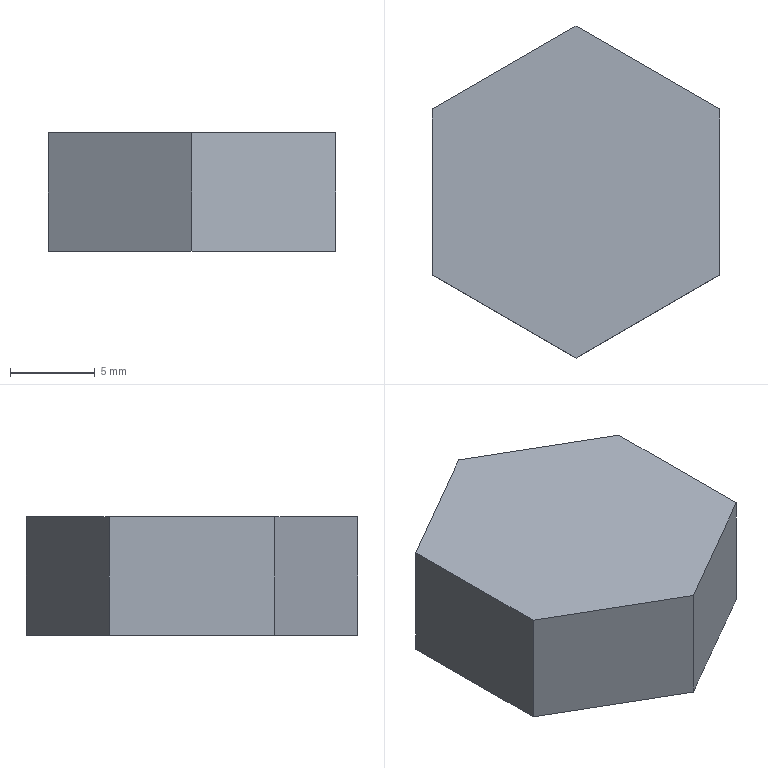Part | SolidWorks | features BaseBody 1 | 1 solid | 15 faces | box 17 x 19.63 x 7 mm | volume 818.394 mm3 | plane 15
STEP:
#1=CARTESIAN_POINT('',(-7.,-4.041,5.5));
#2=VERTEX_POINT('',#1);
#3=CARTESIAN_POINT('',(0.,-8.083,5.5));
#4=VERTEX_POINT('',#3);
#5=CARTESIAN_POINT('',(-7.75,-3.608,5.5));
#6=DIRECTION('',(0.866,-0.5,0.));
#7=VECTOR('',#6,1000.);
#8=LINE('',#5,#7);
#9=EDGE_CURVE('',#2,#4,#8,.T.);
#10=ORIENTED_EDGE('',*,*,#9,.F.);
#11=CARTESIAN_POINT('',(-7.,4.041,5.5));
#12=VERTEX_POINT('',#11);
#13=CARTESIAN_POINT('',(-7.,4.907,5.5));
#14=DIRECTION('',(0.,-1.,0.));
#15=VECTOR('',#14,1000.);
#16=LINE('',#13,#15);
#17=EDGE_CURVE('',#12,#2,#16,.T.);
#18=ORIENTED_EDGE('',*,*,#17,.F.);
#19=CARTESIAN_POINT('',(0.,8.083,5.5));
#20=VERTEX_POINT('',#19);
#21=CARTESIAN_POINT('',(0.75,8.516,5.5));
#22=DIRECTION('',(-0.866,-0.5,0.));
#23=VECTOR('',#22,1000.);
#24=LINE('',#21,#23);
#25=EDGE_CURVE('',#20,#12,#24,.T.);
#26=ORIENTED_EDGE('',*,*,#25,.F.);
#27=CARTESIAN_POINT('',(7.,4.041,5.5));
#28=VERTEX_POINT('',#27);
#29=CARTESIAN_POINT('',(7.75,3.608,5.5));
#30=DIRECTION('',(-0.866,0.5,0.));
#31=VECTOR('',#30,1000.);
#32=LINE('',#29,#31);
#33=EDGE_CURVE('',#28,#20,#32,.T.);
#34=ORIENTED_EDGE('',*,*,#33,.F.);
#35=CARTESIAN_POINT('',(7.,-4.041,5.5));
#36=VERTEX_POINT('',#35);
#37=CARTESIAN_POINT('',(7.,-4.907,5.5));
#38=DIRECTION('',(0.,1.,0.));
#39=VECTOR('',#38,1000.);
#40=LINE('',#37,#39);
#41=EDGE_CURVE('',#36,#28,#40,.T.);
#42=ORIENTED_EDGE('',*,*,#41,.F.);
#43=CARTESIAN_POINT('',(-0.75,-8.516,5.5));
#44=DIRECTION('',(0.866,0.5,0.));
#45=VECTOR('',#44,1000.);
#46=LINE('',#43,#45);
#47=EDGE_CURVE('',#4,#36,#46,.T.);
#48=ORIENTED_EDGE('',*,*,#47,.F.);
#49=EDGE_LOOP('',(#10,#18,#26,#34,#42,#48));
#50=FACE_OUTER_BOUND('',#49,.T.);
#51=CARTESIAN_POINT('',(0.,0.,5.5));
#52=DIRECTION('',(0.,0.,1.));
#53=DIRECTION('',(1.,0.,0.));
#54=AXIS2_PLACEMENT_3D('',#51,#52,#53);
#55=PLANE('',#54);
#56=ADVANCED_FACE('',(#50),#55,.F.);
#57=CARTESIAN_POINT('',(-7.,4.041,0.));
#58=VERTEX_POINT('',#57);
#59=CARTESIAN_POINT('',(-7.,-4.041,0.));
#60=VERTEX_POINT('',#59);
#61=CARTESIAN_POINT('',(-7.,4.907,0.));
#62=DIRECTION('',(0.,-1.,0.));
#63=VECTOR('',#62,1000.);
#64=LINE('',#61,#63);
#65=EDGE_CURVE('',#58,#60,#64,.T.);
#66=ORIENTED_EDGE('',*,*,#65,.F.);
#67=CARTESIAN_POINT('',(-7.,4.041,7.));
#68=DIRECTION('',(0.,0.,-1.));
#69=VECTOR('',#68,1000.);
#70=LINE('',#67,#69);
#71=EDGE_CURVE('',#12,#58,#70,.T.);
#72=ORIENTED_EDGE('',*,*,#71,.F.);
#73=ORIENTED_EDGE('',*,*,#17,.T.);
#74=CARTESIAN_POINT('',(-7.,-4.041,7.));
#75=DIRECTION('',(0.,0.,-1.));
#76=VECTOR('',#75,1000.);
#77=LINE('',#74,#76);
#78=EDGE_CURVE('',#2,#60,#77,.T.);
#79=ORIENTED_EDGE('',*,*,#78,.T.);
#80=EDGE_LOOP('',(#66,#72,#73,#79));
#81=FACE_OUTER_BOUND('',#80,.T.);
#82=CARTESIAN_POINT('',(-7.,4.907,7.));
#83=DIRECTION('',(1.,0.,0.));
#84=DIRECTION('',(0.,1.,0.));
#85=AXIS2_PLACEMENT_3D('',#82,#83,#84);
#86=PLANE('',#85);
#87=ADVANCED_FACE('',(#81),#86,.T.);
#88=CARTESIAN_POINT('',(0.,8.083,0.));
#89=VERTEX_POINT('',#88);
#90=CARTESIAN_POINT('',(0.75,8.516,0.));
#91=DIRECTION('',(-0.866,-0.5,0.));
#92=VECTOR('',#91,1000.);
#93=LINE('',#90,#92);
#94=EDGE_CURVE('',#89,#58,#93,.T.);
#95=ORIENTED_EDGE('',*,*,#94,.F.);
#96=CARTESIAN_POINT('',(0.,8.083,7.));
#97=DIRECTION('',(0.,0.,-1.));
#98=VECTOR('',#97,1000.);
#99=LINE('',#96,#98);
#100=EDGE_CURVE('',#20,#89,#99,.T.);
#101=ORIENTED_EDGE('',*,*,#100,.F.);
#102=ORIENTED_EDGE('',*,*,#25,.T.);
#103=ORIENTED_EDGE('',*,*,#71,.T.);
#104=EDGE_LOOP('',(#95,#101,#102,#103));
#105=FACE_OUTER_BOUND('',#104,.T.);
#106=CARTESIAN_POINT('',(0.75,8.516,7.));
#107=DIRECTION('',(0.5,-0.866,0.));
#108=DIRECTION('',(0.,0.,-1.));
#109=AXIS2_PLACEMENT_3D('',#106,#107,#108);
#110=PLANE('',#109);
#111=ADVANCED_FACE('',(#105),#110,.T.);
#112=CARTESIAN_POINT('',(7.,4.041,0.));
#113=VERTEX_POINT('',#112);
#114=CARTESIAN_POINT('',(7.75,3.608,0.));
#115=DIRECTION('',(-0.866,0.5,0.));
#116=VECTOR('',#115,1000.);
#117=LINE('',#114,#116);
#118=EDGE_CURVE('',#113,#89,#117,.T.);
#119=ORIENTED_EDGE('',*,*,#118,.F.);
#120=CARTESIAN_POINT('',(7.,4.041,7.));
#121=DIRECTION('',(0.,0.,-1.));
#122=VECTOR('',#121,1000.);
#123=LINE('',#120,#122);
#124=EDGE_CURVE('',#28,#113,#123,.T.);
#125=ORIENTED_EDGE('',*,*,#124,.F.);
#126=ORIENTED_EDGE('',*,*,#33,.T.);
#127=ORIENTED_EDGE('',*,*,#100,.T.);
#128=EDGE_LOOP('',(#119,#125,#126,#127));
#129=FACE_OUTER_BOUND('',#128,.T.);
#130=CARTESIAN_POINT('',(7.75,3.608,7.));
#131=DIRECTION('',(-0.5,-0.866,0.));
#132=DIRECTION('',(-0.866,0.5,0.));
#133=AXIS2_PLACEMENT_3D('',#130,#131,#132);
#134=PLANE('',#133);
#135=ADVANCED_FACE('',(#129),#134,.T.);
#136=CARTESIAN_POINT('',(7.,-4.041,0.));
#137=VERTEX_POINT('',#136);
#138=CARTESIAN_POINT('',(7.,-4.907,0.));
#139=DIRECTION('',(0.,1.,0.));
#140=VECTOR('',#139,1000.);
#141=LINE('',#138,#140);
#142=EDGE_CURVE('',#137,#113,#141,.T.);
#143=ORIENTED_EDGE('',*,*,#142,.F.);
#144=CARTESIAN_POINT('',(7.,-4.041,7.));
#145=DIRECTION('',(0.,0.,-1.));
#146=VECTOR('',#145,1000.);
#147=LINE('',#144,#146);
#148=EDGE_CURVE('',#36,#137,#147,.T.);
#149=ORIENTED_EDGE('',*,*,#148,.F.);
#150=ORIENTED_EDGE('',*,*,#41,.T.);
#151=ORIENTED_EDGE('',*,*,#124,.T.);
#152=EDGE_LOOP('',(#143,#149,#150,#151));
#153=FACE_OUTER_BOUND('',#152,.T.);
#154=CARTESIAN_POINT('',(7.,-4.907,7.));
#155=DIRECTION('',(-1.,0.,0.));
#156=DIRECTION('',(0.,0.,1.));
#157=AXIS2_PLACEMENT_3D('',#154,#155,#156);
#158=PLANE('',#157);
#159=ADVANCED_FACE('',(#153),#158,.T.);
#160=CARTESIAN_POINT('',(0.,-8.083,0.));
#161=VERTEX_POINT('',#160);
#162=CARTESIAN_POINT('',(-0.75,-8.516,0.));
#163=DIRECTION('',(0.866,0.5,0.));
#164=VECTOR('',#163,1000.);
#165=LINE('',#162,#164);
#166=EDGE_CURVE('',#161,#137,#165,.T.);
#167=ORIENTED_EDGE('',*,*,#166,.F.);
#168=CARTESIAN_POINT('',(0.,-8.083,7.));
#169=DIRECTION('',(0.,0.,-1.));
#170=VECTOR('',#169,1000.);
#171=LINE('',#168,#170);
#172=EDGE_CURVE('',#4,#161,#171,.T.);
#173=ORIENTED_EDGE('',*,*,#172,.F.);
#174=ORIENTED_EDGE('',*,*,#47,.T.);
#175=ORIENTED_EDGE('',*,*,#148,.T.);
#176=EDGE_LOOP('',(#167,#173,#174,#175));
#177=FACE_OUTER_BOUND('',#176,.T.);
#178=CARTESIAN_POINT('',(-0.75,-8.516,7.));
#179=DIRECTION('',(-0.5,0.866,0.));
#180=DIRECTION('',(0.,0.,1.));
#181=AXIS2_PLACEMENT_3D('',#178,#179,#180);
#182=PLANE('',#181);
#183=ADVANCED_FACE('',(#177),#182,.T.);
#184=CARTESIAN_POINT('',(-7.75,-3.608,0.));
#185=DIRECTION('',(0.866,-0.5,0.));
#186=VECTOR('',#185,1000.);
#187=LINE('',#184,#186);
#188=EDGE_CURVE('',#60,#161,#187,.T.);
#189=ORIENTED_EDGE('',*,*,#188,.F.);
#190=ORIENTED_EDGE('',*,*,#78,.F.);
#191=ORIENTED_EDGE('',*,*,#9,.T.);
#192=ORIENTED_EDGE('',*,*,#172,.T.);
#193=EDGE_LOOP('',(#189,#190,#191,#192));
#194=FACE_OUTER_BOUND('',#193,.T.);
#195=CARTESIAN_POINT('',(-7.75,-3.608,7.));
#196=DIRECTION('',(0.5,0.866,0.));
#197=DIRECTION('',(0.,0.,-1.));
#198=AXIS2_PLACEMENT_3D('',#195,#196,#197);
#199=PLANE('',#198);
#200=ADVANCED_FACE('',(#194),#199,.T.);
#201=ORIENTED_EDGE('',*,*,#65,.T.);
#202=ORIENTED_EDGE('',*,*,#188,.T.);
#203=ORIENTED_EDGE('',*,*,#166,.T.);
#204=ORIENTED_EDGE('',*,*,#142,.T.);
#205=ORIENTED_EDGE('',*,*,#118,.T.);
#206=ORIENTED_EDGE('',*,*,#94,.T.);
#207=EDGE_LOOP('',(#201,#202,#203,#204,#205,#206));
#208=FACE_BOUND('',#207,.T.);
#209=CARTESIAN_POINT('',(-8.5,-4.907,0.));
#210=VERTEX_POINT('',#209);
#211=CARTESIAN_POINT('',(0.,-9.815,0.));
#212=VERTEX_POINT('',#211);
#213=CARTESIAN_POINT('',(-8.5,-4.907,0.));
#214=DIRECTION('',(0.866,-0.5,0.));
#215=VECTOR('',#214,1000.);
#216=LINE('',#213,#215);
#217=EDGE_CURVE('',#210,#212,#216,.T.);
#218=ORIENTED_EDGE('',*,*,#217,.F.);
#219=CARTESIAN_POINT('',(-8.5,4.907,0.));
#220=VERTEX_POINT('',#219);
#221=CARTESIAN_POINT('',(-8.5,4.907,0.));
#222=DIRECTION('',(0.,-1.,0.));
#223=VECTOR('',#222,1000.);
#224=LINE('',#221,#223);
#225=EDGE_CURVE('',#220,#210,#224,.T.);
#226=ORIENTED_EDGE('',*,*,#225,.F.);
#227=CARTESIAN_POINT('',(0.,9.815,0.));
#228=VERTEX_POINT('',#227);
#229=CARTESIAN_POINT('',(0.,9.815,0.));
#230=DIRECTION('',(-0.866,-0.5,0.));
#231=VECTOR('',#230,1000.);
#232=LINE('',#229,#231);
#233=EDGE_CURVE('',#228,#220,#232,.T.);
#234=ORIENTED_EDGE('',*,*,#233,.F.);
#235=CARTESIAN_POINT('',(8.5,4.907,0.));
#236=VERTEX_POINT('',#235);
#237=CARTESIAN_POINT('',(8.5,4.907,0.));
#238=DIRECTION('',(-0.866,0.5,0.));
#239=VECTOR('',#238,1000.);
#240=LINE('',#237,#239);
#241=EDGE_CURVE('',#236,#228,#240,.T.);
#242=ORIENTED_EDGE('',*,*,#241,.F.);
#243=CARTESIAN_POINT('',(8.5,-4.907,0.));
#244=VERTEX_POINT('',#243);
#245=CARTESIAN_POINT('',(8.5,-4.907,0.));
#246=DIRECTION('',(0.,1.,0.));
#247=VECTOR('',#246,1000.);
#248=LINE('',#245,#247);
#249=EDGE_CURVE('',#244,#236,#248,.T.);
#250=ORIENTED_EDGE('',*,*,#249,.F.);
#251=CARTESIAN_POINT('',(0.,-9.815,0.));
#252=DIRECTION('',(0.866,0.5,0.));
#253=VECTOR('',#252,1000.);
#254=LINE('',#251,#253);
#255=EDGE_CURVE('',#212,#244,#254,.T.);
#256=ORIENTED_EDGE('',*,*,#255,.F.);
#257=EDGE_LOOP('',(#218,#226,#234,#242,#250,#256));
#258=FACE_OUTER_BOUND('',#257,.T.);
#259=CARTESIAN_POINT('',(0.,0.,0.));
#260=DIRECTION('',(0.,0.,1.));
#261=DIRECTION('',(1.,0.,0.));
#262=AXIS2_PLACEMENT_3D('',#259,#260,#261);
#263=PLANE('',#262);
#264=ADVANCED_FACE('',(#208,#258),#263,.F.);
#265=CARTESIAN_POINT('',(-8.5,-4.907,7.));
#266=VERTEX_POINT('',#265);
#267=CARTESIAN_POINT('',(0.,-9.815,7.));
#268=VERTEX_POINT('',#267);
#269=CARTESIAN_POINT('',(-8.5,-4.907,7.));
#270=DIRECTION('',(0.866,-0.5,0.));
#271=VECTOR('',#270,1000.);
#272=LINE('',#269,#271);
#273=EDGE_CURVE('',#266,#268,#272,.T.);
#274=ORIENTED_EDGE('',*,*,#273,.T.);
#275=CARTESIAN_POINT('',(8.5,-4.907,7.));
#276=VERTEX_POINT('',#275);
#277=CARTESIAN_POINT('',(0.,-9.815,7.));
#278=DIRECTION('',(0.866,0.5,0.));
#279=VECTOR('',#278,1000.);
#280=LINE('',#277,#279);
#281=EDGE_CURVE('',#268,#276,#280,.T.);
#282=ORIENTED_EDGE('',*,*,#281,.T.);
#283=CARTESIAN_POINT('',(8.5,4.907,7.));
#284=VERTEX_POINT('',#283);
#285=CARTESIAN_POINT('',(8.5,-4.907,7.));
#286=DIRECTION('',(0.,1.,0.));
#287=VECTOR('',#286,1000.);
#288=LINE('',#285,#287);
#289=EDGE_CURVE('',#276,#284,#288,.T.);
#290=ORIENTED_EDGE('',*,*,#289,.T.);
#291=CARTESIAN_POINT('',(0.,9.815,7.));
#292=VERTEX_POINT('',#291);
#293=CARTESIAN_POINT('',(8.5,4.907,7.));
#294=DIRECTION('',(-0.866,0.5,0.));
#295=VECTOR('',#294,1000.);
#296=LINE('',#293,#295);
#297=EDGE_CURVE('',#284,#292,#296,.T.);
#298=ORIENTED_EDGE('',*,*,#297,.T.);
#299=CARTESIAN_POINT('',(-8.5,4.907,7.));
#300=VERTEX_POINT('',#299);
#301=CARTESIAN_POINT('',(0.,9.815,7.));
#302=DIRECTION('',(-0.866,-0.5,0.));
#303=VECTOR('',#302,1000.);
#304=LINE('',#301,#303);
#305=EDGE_CURVE('',#292,#300,#304,.T.);
#306=ORIENTED_EDGE('',*,*,#305,.T.);
#307=CARTESIAN_POINT('',(-8.5,4.907,7.));
#308=DIRECTION('',(0.,-1.,0.));
#309=VECTOR('',#308,1000.);
#310=LINE('',#307,#309);
#311=EDGE_CURVE('',#300,#266,#310,.T.);
#312=ORIENTED_EDGE('',*,*,#311,.T.);
#313=EDGE_LOOP('',(#274,#282,#290,#298,#306,#312));
#314=FACE_OUTER_BOUND('',#313,.T.);
#315=CARTESIAN_POINT('',(0.,0.,7.));
#316=DIRECTION('',(0.,0.,1.));
#317=DIRECTION('',(1.,0.,0.));
#318=AXIS2_PLACEMENT_3D('',#315,#316,#317);
#319=PLANE('',#318);
#320=ADVANCED_FACE('',(#314),#319,.T.);
#321=ORIENTED_EDGE('',*,*,#225,.T.);
#322=CARTESIAN_POINT('',(-8.5,-4.907,7.));
#323=DIRECTION('',(0.,0.,-1.));
#324=VECTOR('',#323,1000.);
#325=LINE('',#322,#324);
#326=EDGE_CURVE('',#266,#210,#325,.T.);
#327=ORIENTED_EDGE('',*,*,#326,.F.);
#328=ORIENTED_EDGE('',*,*,#311,.F.);
#329=CARTESIAN_POINT('',(-8.5,4.907,7.));
#330=DIRECTION('',(0.,0.,-1.));
#331=VECTOR('',#330,1000.);
#332=LINE('',#329,#331);
#333=EDGE_CURVE('',#300,#220,#332,.T.);
#334=ORIENTED_EDGE('',*,*,#333,.T.);
#335=EDGE_LOOP('',(#321,#327,#328,#334));
#336=FACE_OUTER_BOUND('',#335,.T.);
#337=CARTESIAN_POINT('',(-8.5,4.907,7.));
#338=DIRECTION('',(1.,0.,0.));
#339=DIRECTION('',(0.,1.,0.));
#340=AXIS2_PLACEMENT_3D('',#337,#338,#339);
#341=PLANE('',#340);
#342=ADVANCED_FACE('',(#336),#341,.F.);
#343=ORIENTED_EDGE('',*,*,#233,.T.);
#344=ORIENTED_EDGE('',*,*,#333,.F.);
#345=ORIENTED_EDGE('',*,*,#305,.F.);
#346=CARTESIAN_POINT('',(0.,9.815,7.));
#347=DIRECTION('',(0.,0.,-1.));
#348=VECTOR('',#347,1000.);
#349=LINE('',#346,#348);
#350=EDGE_CURVE('',#292,#228,#349,.T.);
#351=ORIENTED_EDGE('',*,*,#350,.T.);
#352=EDGE_LOOP('',(#343,#344,#345,#351));
#353=FACE_OUTER_BOUND('',#352,.T.);
#354=CARTESIAN_POINT('',(0.,9.815,7.));
#355=DIRECTION('',(0.5,-0.866,0.));
#356=DIRECTION('',(0.,0.,-1.));
#357=AXIS2_PLACEMENT_3D('',#354,#355,#356);
#358=PLANE('',#357);
#359=ADVANCED_FACE('',(#353),#358,.F.);
#360=ORIENTED_EDGE('',*,*,#241,.T.);
#361=ORIENTED_EDGE('',*,*,#350,.F.);
#362=ORIENTED_EDGE('',*,*,#297,.F.);
#363=CARTESIAN_POINT('',(8.5,4.907,7.));
#364=DIRECTION('',(0.,0.,-1.));
#365=VECTOR('',#364,1000.);
#366=LINE('',#363,#365);
#367=EDGE_CURVE('',#284,#236,#366,.T.);
#368=ORIENTED_EDGE('',*,*,#367,.T.);
#369=EDGE_LOOP('',(#360,#361,#362,#368));
#370=FACE_OUTER_BOUND('',#369,.T.);
#371=CARTESIAN_POINT('',(8.5,4.907,7.));
#372=DIRECTION('',(-0.5,-0.866,0.));
#373=DIRECTION('',(-0.866,0.5,0.));
#374=AXIS2_PLACEMENT_3D('',#371,#372,#373);
#375=PLANE('',#374);
#376=ADVANCED_FACE('',(#370),#375,.F.);
#377=ORIENTED_EDGE('',*,*,#249,.T.);
#378=ORIENTED_EDGE('',*,*,#367,.F.);
#379=ORIENTED_EDGE('',*,*,#289,.F.);
#380=CARTESIAN_POINT('',(8.5,-4.907,7.));
#381=DIRECTION('',(0.,0.,-1.));
#382=VECTOR('',#381,1000.);
#383=LINE('',#380,#382);
#384=EDGE_CURVE('',#276,#244,#383,.T.);
#385=ORIENTED_EDGE('',*,*,#384,.T.);
#386=EDGE_LOOP('',(#377,#378,#379,#385));
#387=FACE_OUTER_BOUND('',#386,.T.);
#388=CARTESIAN_POINT('',(8.5,-4.907,7.));
#389=DIRECTION('',(-1.,0.,0.));
#390=DIRECTION('',(0.,0.,1.));
#391=AXIS2_PLACEMENT_3D('',#388,#389,#390);
#392=PLANE('',#391);
#393=ADVANCED_FACE('',(#387),#392,.F.);
#394=ORIENTED_EDGE('',*,*,#255,.T.);
#395=ORIENTED_EDGE('',*,*,#384,.F.);
#396=ORIENTED_EDGE('',*,*,#281,.F.);
#397=CARTESIAN_POINT('',(0.,-9.815,7.));
#398=DIRECTION('',(0.,0.,-1.));
#399=VECTOR('',#398,1000.);
#400=LINE('',#397,#399);
#401=EDGE_CURVE('',#268,#212,#400,.T.);
#402=ORIENTED_EDGE('',*,*,#401,.T.);
#403=EDGE_LOOP('',(#394,#395,#396,#402));
#404=FACE_OUTER_BOUND('',#403,.T.);
#405=CARTESIAN_POINT('',(0.,-9.815,7.));
#406=DIRECTION('',(-0.5,0.866,0.));
#407=DIRECTION('',(0.,0.,1.));
#408=AXIS2_PLACEMENT_3D('',#405,#406,#407);
#409=PLANE('',#408);
#410=ADVANCED_FACE('',(#404),#409,.F.);
#411=ORIENTED_EDGE('',*,*,#217,.T.);
#412=ORIENTED_EDGE('',*,*,#401,.F.);
#413=ORIENTED_EDGE('',*,*,#273,.F.);
#414=ORIENTED_EDGE('',*,*,#326,.T.);
#415=EDGE_LOOP('',(#411,#412,#413,#414));
#416=FACE_OUTER_BOUND('',#415,.T.);
#417=CARTESIAN_POINT('',(-8.5,-4.907,7.));
#418=DIRECTION('',(0.5,0.866,0.));
#419=DIRECTION('',(0.,0.,-1.));
#420=AXIS2_PLACEMENT_3D('',#417,#418,#419);
#421=PLANE('',#420);
#422=ADVANCED_FACE('',(#416),#421,.F.);
#423=CLOSED_SHELL('',(#56,#87,#111,#135,#159,#183,#200,#264,#320,#342,#359,#376,#393,#410,#422));
#424=MANIFOLD_SOLID_BREP('',#423);
#425=CARTESIAN_POINT('',(0.,0.,0.));
#426=DIRECTION('',(0.,0.,1.));
#427=DIRECTION('',(1.,0.,0.));
#428=AXIS2_PLACEMENT_3D('',#425,#426,#427);
#429=(LENGTH_UNIT()NAMED_UNIT(*)SI_UNIT(.MILLI.,.METRE.));
#430=UNCERTAINTY_MEASURE_WITH_UNIT(LENGTH_MEASURE(0.00001),#429,'','');
#431=(NAMED_UNIT(*)PLANE_ANGLE_UNIT()SI_UNIT($,.RADIAN.));
#432=(NAMED_UNIT(*)SI_UNIT($,.STERADIAN.)SOLID_ANGLE_UNIT());
#433=(GEOMETRIC_REPRESENTATION_CONTEXT(3)GLOBAL_UNCERTAINTY_ASSIGNED_CONTEXT((#430))GLOBAL_UNIT_ASSIGNED_CONTEXT((#429,#431,#432))REPRESENTATION_CONTEXT('',''));
#434=ADVANCED_BREP_SHAPE_REPRESENTATION('',(#424,#428),#433);